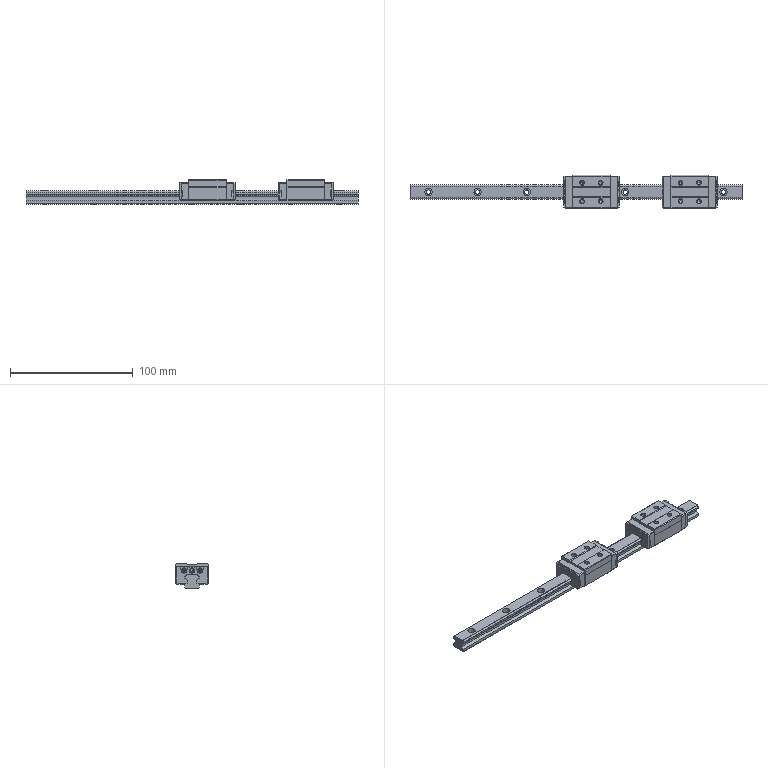Part | NX | 3 solids | 797 faces | box 270 x 27 x 20 mm | volume 58637 mm3 | plane 465 | cylinder 236 | cone 64 | torus 32 | commonest cylinder face diameters 1 x40 2.6 x32 3.5 x30 2 x16 2.24 x16 2.48 x16